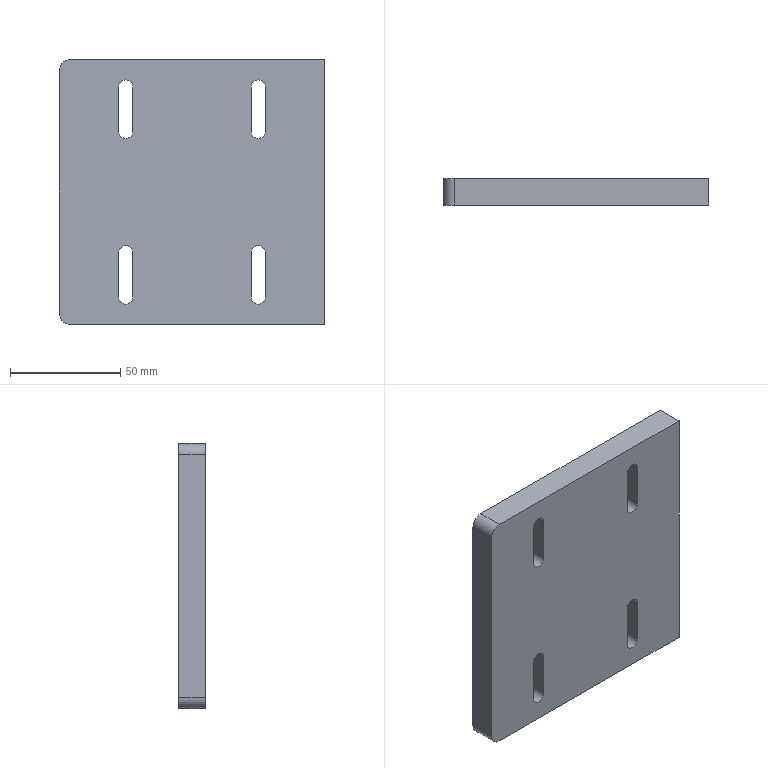Part | STEP file | PN_0023 | 1 solid | 40 faces | box 120 x 12 x 120 mm | volume 163808 mm3 | cylinder 20 | plane 14 | cone 6 | commonest cylinder face diameters 6.5 x12 5 x6 10 x2